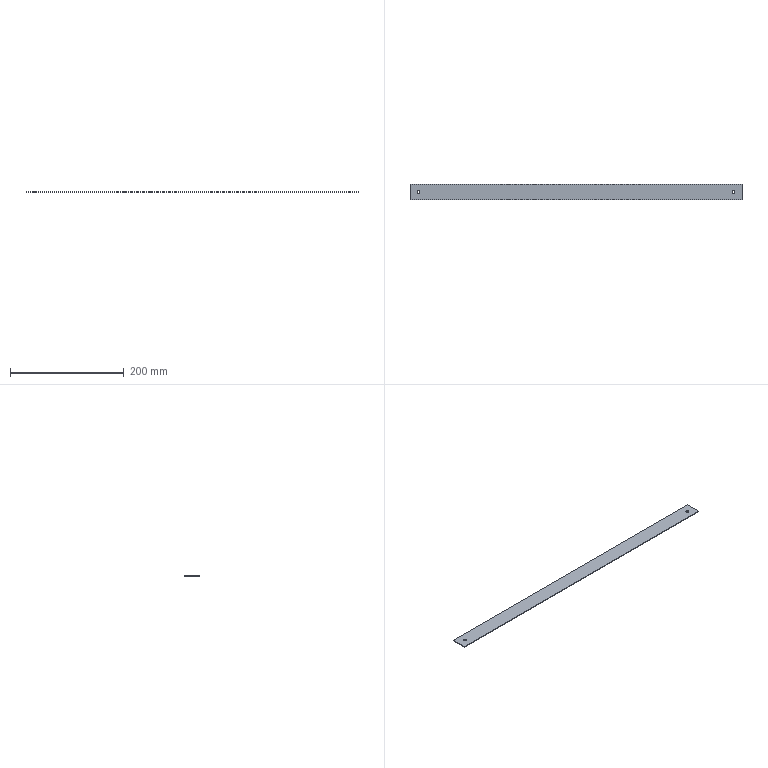Part | SolidWorks | features Extrusion 1, HoleWzd 1 | 1 solid | 10 faces | box 585 x 27.5 x 1.2 mm | volume 19258 mm3 | plane 6 | cylinder 4 | commonest cylinder face diameters 5 x4
STEP:
#1=CARTESIAN_POINT('',(17.5,13.75,0.));
#2=VERTEX_POINT('',#1);
#3=CARTESIAN_POINT('',(12.5,13.75,0.));
#4=VERTEX_POINT('',#3);
#5=CARTESIAN_POINT('',(15.,13.75,0.));
#6=DIRECTION('',(0.,0.,-1.));
#7=DIRECTION('',(-1.,0.,0.));
#8=AXIS2_PLACEMENT_3D('',#5,#6,#7);
#9=CIRCLE('',#8,2.5);
#10=EDGE_CURVE('',#2,#4,#9,.T.);
#11=ORIENTED_EDGE('',*,*,#10,.T.);
#12=CARTESIAN_POINT('',(12.5,13.75,1.2));
#13=VERTEX_POINT('',#12);
#14=CARTESIAN_POINT('',(12.5,13.75,1.2));
#15=DIRECTION('',(0.,0.,1.));
#16=VECTOR('',#15,1000.);
#17=LINE('',#14,#16);
#18=EDGE_CURVE('',#4,#13,#17,.T.);
#19=ORIENTED_EDGE('',*,*,#18,.T.);
#20=CARTESIAN_POINT('',(17.5,13.75,1.2));
#21=VERTEX_POINT('',#20);
#22=CARTESIAN_POINT('',(15.,13.75,1.2));
#23=DIRECTION('',(0.,0.,1.));
#24=DIRECTION('',(1.,0.,0.));
#25=AXIS2_PLACEMENT_3D('',#22,#23,#24);
#26=CIRCLE('',#25,2.5);
#27=EDGE_CURVE('',#13,#21,#26,.T.);
#28=ORIENTED_EDGE('',*,*,#27,.T.);
#29=CARTESIAN_POINT('',(17.5,13.75,1.2));
#30=DIRECTION('',(0.,0.,1.));
#31=VECTOR('',#30,1000.);
#32=LINE('',#29,#31);
#33=EDGE_CURVE('',#2,#21,#32,.T.);
#34=ORIENTED_EDGE('',*,*,#33,.F.);
#35=EDGE_LOOP('',(#11,#19,#28,#34));
#36=FACE_OUTER_BOUND('',#35,.T.);
#37=CARTESIAN_POINT('',(15.,13.75,1.2));
#38=DIRECTION('',(0.,0.,1.));
#39=DIRECTION('',(1.,0.,0.));
#40=AXIS2_PLACEMENT_3D('',#37,#38,#39);
#41=CYLINDRICAL_SURFACE('',#40,2.5);
#42=ADVANCED_FACE('',(#36),#41,.F.);
#43=CARTESIAN_POINT('',(572.5,13.75,0.));
#44=VERTEX_POINT('',#43);
#45=CARTESIAN_POINT('',(567.5,13.75,0.));
#46=VERTEX_POINT('',#45);
#47=CARTESIAN_POINT('',(570.,13.75,0.));
#48=DIRECTION('',(0.,0.,-1.));
#49=DIRECTION('',(-1.,0.,0.));
#50=AXIS2_PLACEMENT_3D('',#47,#48,#49);
#51=CIRCLE('',#50,2.5);
#52=EDGE_CURVE('',#44,#46,#51,.T.);
#53=ORIENTED_EDGE('',*,*,#52,.T.);
#54=CARTESIAN_POINT('',(567.5,13.75,1.2));
#55=VERTEX_POINT('',#54);
#56=CARTESIAN_POINT('',(567.5,13.75,1.2));
#57=DIRECTION('',(0.,0.,1.));
#58=VECTOR('',#57,1000.);
#59=LINE('',#56,#58);
#60=EDGE_CURVE('',#46,#55,#59,.T.);
#61=ORIENTED_EDGE('',*,*,#60,.T.);
#62=CARTESIAN_POINT('',(572.5,13.75,1.2));
#63=VERTEX_POINT('',#62);
#64=CARTESIAN_POINT('',(570.,13.75,1.2));
#65=DIRECTION('',(0.,0.,1.));
#66=DIRECTION('',(1.,0.,0.));
#67=AXIS2_PLACEMENT_3D('',#64,#65,#66);
#68=CIRCLE('',#67,2.5);
#69=EDGE_CURVE('',#55,#63,#68,.T.);
#70=ORIENTED_EDGE('',*,*,#69,.T.);
#71=CARTESIAN_POINT('',(572.5,13.75,1.2));
#72=DIRECTION('',(0.,0.,1.));
#73=VECTOR('',#72,1000.);
#74=LINE('',#71,#73);
#75=EDGE_CURVE('',#44,#63,#74,.T.);
#76=ORIENTED_EDGE('',*,*,#75,.F.);
#77=EDGE_LOOP('',(#53,#61,#70,#76));
#78=FACE_OUTER_BOUND('',#77,.T.);
#79=CARTESIAN_POINT('',(570.,13.75,1.2));
#80=DIRECTION('',(0.,0.,1.));
#81=DIRECTION('',(1.,0.,0.));
#82=AXIS2_PLACEMENT_3D('',#79,#80,#81);
#83=CYLINDRICAL_SURFACE('',#82,2.5);
#84=ADVANCED_FACE('',(#78),#83,.F.);
#85=CARTESIAN_POINT('',(0.,27.5,0.));
#86=VERTEX_POINT('',#85);
#87=CARTESIAN_POINT('',(0.,0.,0.));
#88=VERTEX_POINT('',#87);
#89=CARTESIAN_POINT('',(0.,0.,0.));
#90=DIRECTION('',(0.,-1.,0.));
#91=VECTOR('',#90,1000.);
#92=LINE('',#89,#91);
#93=EDGE_CURVE('',#86,#88,#92,.T.);
#94=ORIENTED_EDGE('',*,*,#93,.T.);
#95=CARTESIAN_POINT('',(0.,0.,1.2));
#96=VERTEX_POINT('',#95);
#97=CARTESIAN_POINT('',(0.,0.,1.2));
#98=DIRECTION('',(0.,0.,-1.));
#99=VECTOR('',#98,1000.);
#100=LINE('',#97,#99);
#101=EDGE_CURVE('',#96,#88,#100,.T.);
#102=ORIENTED_EDGE('',*,*,#101,.F.);
#103=CARTESIAN_POINT('',(0.,27.5,1.2));
#104=VERTEX_POINT('',#103);
#105=CARTESIAN_POINT('',(0.,0.,1.2));
#106=DIRECTION('',(0.,-1.,0.));
#107=VECTOR('',#106,1000.);
#108=LINE('',#105,#107);
#109=EDGE_CURVE('',#104,#96,#108,.T.);
#110=ORIENTED_EDGE('',*,*,#109,.F.);
#111=CARTESIAN_POINT('',(0.,27.5,1.2));
#112=DIRECTION('',(0.,0.,-1.));
#113=VECTOR('',#112,1000.);
#114=LINE('',#111,#113);
#115=EDGE_CURVE('',#104,#86,#114,.T.);
#116=ORIENTED_EDGE('',*,*,#115,.T.);
#117=EDGE_LOOP('',(#94,#102,#110,#116));
#118=FACE_OUTER_BOUND('',#117,.T.);
#119=CARTESIAN_POINT('',(0.,0.,1.2));
#120=DIRECTION('',(1.,0.,0.));
#121=DIRECTION('',(0.,0.,-1.));
#122=AXIS2_PLACEMENT_3D('',#119,#120,#121);
#123=PLANE('',#122);
#124=ADVANCED_FACE('',(#118),#123,.F.);
#125=CARTESIAN_POINT('',(585.,0.,0.));
#126=VERTEX_POINT('',#125);
#127=CARTESIAN_POINT('',(0.,0.,0.));
#128=DIRECTION('',(1.,0.,0.));
#129=VECTOR('',#128,1000.);
#130=LINE('',#127,#129);
#131=EDGE_CURVE('',#88,#126,#130,.T.);
#132=ORIENTED_EDGE('',*,*,#131,.T.);
#133=CARTESIAN_POINT('',(585.,0.,1.2));
#134=VERTEX_POINT('',#133);
#135=CARTESIAN_POINT('',(585.,0.,1.2));
#136=DIRECTION('',(0.,0.,-1.));
#137=VECTOR('',#136,1000.);
#138=LINE('',#135,#137);
#139=EDGE_CURVE('',#134,#126,#138,.T.);
#140=ORIENTED_EDGE('',*,*,#139,.F.);
#141=CARTESIAN_POINT('',(0.,0.,1.2));
#142=DIRECTION('',(1.,0.,0.));
#143=VECTOR('',#142,1000.);
#144=LINE('',#141,#143);
#145=EDGE_CURVE('',#96,#134,#144,.T.);
#146=ORIENTED_EDGE('',*,*,#145,.F.);
#147=ORIENTED_EDGE('',*,*,#101,.T.);
#148=EDGE_LOOP('',(#132,#140,#146,#147));
#149=FACE_OUTER_BOUND('',#148,.T.);
#150=CARTESIAN_POINT('',(0.,0.,1.2));
#151=DIRECTION('',(0.,1.,0.));
#152=DIRECTION('',(0.,0.,1.));
#153=AXIS2_PLACEMENT_3D('',#150,#151,#152);
#154=PLANE('',#153);
#155=ADVANCED_FACE('',(#149),#154,.F.);
#156=CARTESIAN_POINT('',(585.,27.5,0.));
#157=VERTEX_POINT('',#156);
#158=CARTESIAN_POINT('',(585.,0.,0.));
#159=DIRECTION('',(0.,1.,0.));
#160=VECTOR('',#159,1000.);
#161=LINE('',#158,#160);
#162=EDGE_CURVE('',#126,#157,#161,.T.);
#163=ORIENTED_EDGE('',*,*,#162,.T.);
#164=CARTESIAN_POINT('',(585.,27.5,1.2));
#165=VERTEX_POINT('',#164);
#166=CARTESIAN_POINT('',(585.,27.5,1.2));
#167=DIRECTION('',(0.,0.,-1.));
#168=VECTOR('',#167,1000.);
#169=LINE('',#166,#168);
#170=EDGE_CURVE('',#165,#157,#169,.T.);
#171=ORIENTED_EDGE('',*,*,#170,.F.);
#172=CARTESIAN_POINT('',(585.,0.,1.2));
#173=DIRECTION('',(0.,1.,0.));
#174=VECTOR('',#173,1000.);
#175=LINE('',#172,#174);
#176=EDGE_CURVE('',#134,#165,#175,.T.);
#177=ORIENTED_EDGE('',*,*,#176,.F.);
#178=ORIENTED_EDGE('',*,*,#139,.T.);
#179=EDGE_LOOP('',(#163,#171,#177,#178));
#180=FACE_OUTER_BOUND('',#179,.T.);
#181=CARTESIAN_POINT('',(585.,0.,1.2));
#182=DIRECTION('',(-1.,0.,0.));
#183=DIRECTION('',(0.,0.,1.));
#184=AXIS2_PLACEMENT_3D('',#181,#182,#183);
#185=PLANE('',#184);
#186=ADVANCED_FACE('',(#180),#185,.F.);
#187=CARTESIAN_POINT('',(0.,27.5,0.));
#188=DIRECTION('',(-1.,0.,0.));
#189=VECTOR('',#188,1000.);
#190=LINE('',#187,#189);
#191=EDGE_CURVE('',#157,#86,#190,.T.);
#192=ORIENTED_EDGE('',*,*,#191,.T.);
#193=ORIENTED_EDGE('',*,*,#115,.F.);
#194=CARTESIAN_POINT('',(0.,27.5,1.2));
#195=DIRECTION('',(-1.,0.,0.));
#196=VECTOR('',#195,1000.);
#197=LINE('',#194,#196);
#198=EDGE_CURVE('',#165,#104,#197,.T.);
#199=ORIENTED_EDGE('',*,*,#198,.F.);
#200=ORIENTED_EDGE('',*,*,#170,.T.);
#201=EDGE_LOOP('',(#192,#193,#199,#200));
#202=FACE_OUTER_BOUND('',#201,.T.);
#203=CARTESIAN_POINT('',(0.,27.5,1.2));
#204=DIRECTION('',(0.,-1.,0.));
#205=DIRECTION('',(0.,0.,-1.));
#206=AXIS2_PLACEMENT_3D('',#203,#204,#205);
#207=PLANE('',#206);
#208=ADVANCED_FACE('',(#202),#207,.F.);
#209=CARTESIAN_POINT('',(15.,13.75,1.2));
#210=DIRECTION('',(0.,0.,1.));
#211=DIRECTION('',(1.,0.,0.));
#212=AXIS2_PLACEMENT_3D('',#209,#210,#211);
#213=CIRCLE('',#212,2.5);
#214=EDGE_CURVE('',#21,#13,#213,.T.);
#215=ORIENTED_EDGE('',*,*,#214,.F.);
#216=ORIENTED_EDGE('',*,*,#27,.F.);
#217=EDGE_LOOP('',(#215,#216));
#218=FACE_BOUND('',#217,.T.);
#219=CARTESIAN_POINT('',(570.,13.75,1.2));
#220=DIRECTION('',(0.,0.,1.));
#221=DIRECTION('',(1.,0.,0.));
#222=AXIS2_PLACEMENT_3D('',#219,#220,#221);
#223=CIRCLE('',#222,2.5);
#224=EDGE_CURVE('',#63,#55,#223,.T.);
#225=ORIENTED_EDGE('',*,*,#224,.F.);
#226=ORIENTED_EDGE('',*,*,#69,.F.);
#227=EDGE_LOOP('',(#225,#226));
#228=FACE_BOUND('',#227,.T.);
#229=ORIENTED_EDGE('',*,*,#109,.T.);
#230=ORIENTED_EDGE('',*,*,#145,.T.);
#231=ORIENTED_EDGE('',*,*,#176,.T.);
#232=ORIENTED_EDGE('',*,*,#198,.T.);
#233=EDGE_LOOP('',(#229,#230,#231,#232));
#234=FACE_OUTER_BOUND('',#233,.T.);
#235=CARTESIAN_POINT('',(0.,0.,1.2));
#236=DIRECTION('',(0.,0.,-1.));
#237=DIRECTION('',(-1.,0.,0.));
#238=AXIS2_PLACEMENT_3D('',#235,#236,#237);
#239=PLANE('',#238);
#240=ADVANCED_FACE('',(#218,#228,#234),#239,.F.);
#241=ORIENTED_EDGE('',*,*,#10,.F.);
#242=CARTESIAN_POINT('',(15.,13.75,0.));
#243=DIRECTION('',(0.,0.,-1.));
#244=DIRECTION('',(-1.,0.,0.));
#245=AXIS2_PLACEMENT_3D('',#242,#243,#244);
#246=CIRCLE('',#245,2.5);
#247=EDGE_CURVE('',#4,#2,#246,.T.);
#248=ORIENTED_EDGE('',*,*,#247,.F.);
#249=EDGE_LOOP('',(#241,#248));
#250=FACE_BOUND('',#249,.T.);
#251=ORIENTED_EDGE('',*,*,#52,.F.);
#252=CARTESIAN_POINT('',(570.,13.75,0.));
#253=DIRECTION('',(0.,0.,-1.));
#254=DIRECTION('',(-1.,0.,0.));
#255=AXIS2_PLACEMENT_3D('',#252,#253,#254);
#256=CIRCLE('',#255,2.5);
#257=EDGE_CURVE('',#46,#44,#256,.T.);
#258=ORIENTED_EDGE('',*,*,#257,.F.);
#259=EDGE_LOOP('',(#251,#258));
#260=FACE_BOUND('',#259,.T.);
#261=ORIENTED_EDGE('',*,*,#93,.F.);
#262=ORIENTED_EDGE('',*,*,#191,.F.);
#263=ORIENTED_EDGE('',*,*,#162,.F.);
#264=ORIENTED_EDGE('',*,*,#131,.F.);
#265=EDGE_LOOP('',(#261,#262,#263,#264));
#266=FACE_OUTER_BOUND('',#265,.T.);
#267=CARTESIAN_POINT('',(0.,0.,0.));
#268=DIRECTION('',(0.,0.,-1.));
#269=DIRECTION('',(-1.,0.,0.));
#270=AXIS2_PLACEMENT_3D('',#267,#268,#269);
#271=PLANE('',#270);
#272=ADVANCED_FACE('',(#250,#260,#266),#271,.T.);
#273=ORIENTED_EDGE('',*,*,#60,.F.);
#274=ORIENTED_EDGE('',*,*,#257,.T.);
#275=ORIENTED_EDGE('',*,*,#75,.T.);
#276=ORIENTED_EDGE('',*,*,#224,.T.);
#277=EDGE_LOOP('',(#273,#274,#275,#276));
#278=FACE_OUTER_BOUND('',#277,.T.);
#279=CARTESIAN_POINT('',(570.,13.75,1.2));
#280=DIRECTION('',(0.,0.,1.));
#281=DIRECTION('',(1.,0.,0.));
#282=AXIS2_PLACEMENT_3D('',#279,#280,#281);
#283=CYLINDRICAL_SURFACE('',#282,2.5);
#284=ADVANCED_FACE('',(#278),#283,.F.);
#285=ORIENTED_EDGE('',*,*,#18,.F.);
#286=ORIENTED_EDGE('',*,*,#247,.T.);
#287=ORIENTED_EDGE('',*,*,#33,.T.);
#288=ORIENTED_EDGE('',*,*,#214,.T.);
#289=EDGE_LOOP('',(#285,#286,#287,#288));
#290=FACE_OUTER_BOUND('',#289,.T.);
#291=CARTESIAN_POINT('',(15.,13.75,1.2));
#292=DIRECTION('',(0.,0.,1.));
#293=DIRECTION('',(1.,0.,0.));
#294=AXIS2_PLACEMENT_3D('',#291,#292,#293);
#295=CYLINDRICAL_SURFACE('',#294,2.5);
#296=ADVANCED_FACE('',(#290),#295,.F.);
#297=CLOSED_SHELL('',(#42,#84,#124,#155,#186,#208,#240,#272,#284,#296));
#298=MANIFOLD_SOLID_BREP('',#297);
#299=CARTESIAN_POINT('',(0.,0.,0.));
#300=DIRECTION('',(0.,0.,1.));
#301=DIRECTION('',(1.,0.,0.));
#302=AXIS2_PLACEMENT_3D('',#299,#300,#301);
#303=(LENGTH_UNIT()NAMED_UNIT(*)SI_UNIT(.MILLI.,.METRE.));
#304=UNCERTAINTY_MEASURE_WITH_UNIT(LENGTH_MEASURE(0.00001),#303,'','');
#305=(NAMED_UNIT(*)PLANE_ANGLE_UNIT()SI_UNIT($,.RADIAN.));
#306=(NAMED_UNIT(*)SI_UNIT($,.STERADIAN.)SOLID_ANGLE_UNIT());
#307=(GEOMETRIC_REPRESENTATION_CONTEXT(3)GLOBAL_UNCERTAINTY_ASSIGNED_CONTEXT((#304))GLOBAL_UNIT_ASSIGNED_CONTEXT((#303,#305,#306))REPRESENTATION_CONTEXT('',''));
#308=ADVANCED_BREP_SHAPE_REPRESENTATION('',(#298,#302),#307);